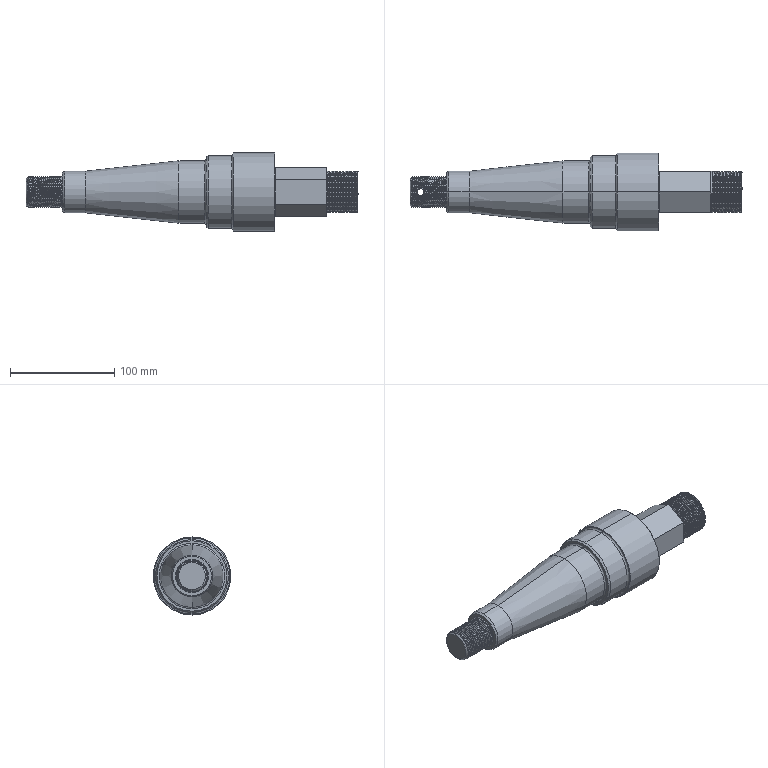Part | SolidWorks | features Chamfer 4, Fillet 4, ICE 3, SweepThread 2, Cut 1, RefAxis 1, Revolution 1 | 1 solid | 153 faces | box 319 x 75 x 75 mm | volume 683914 mm3 | cylinder 84 | plane 27 | spline 25 | cone 11 | torus 6 | commonest cylinder face diameters 40 x43 30 x33 6.3 x2 60 x2 70 x2 75 x2